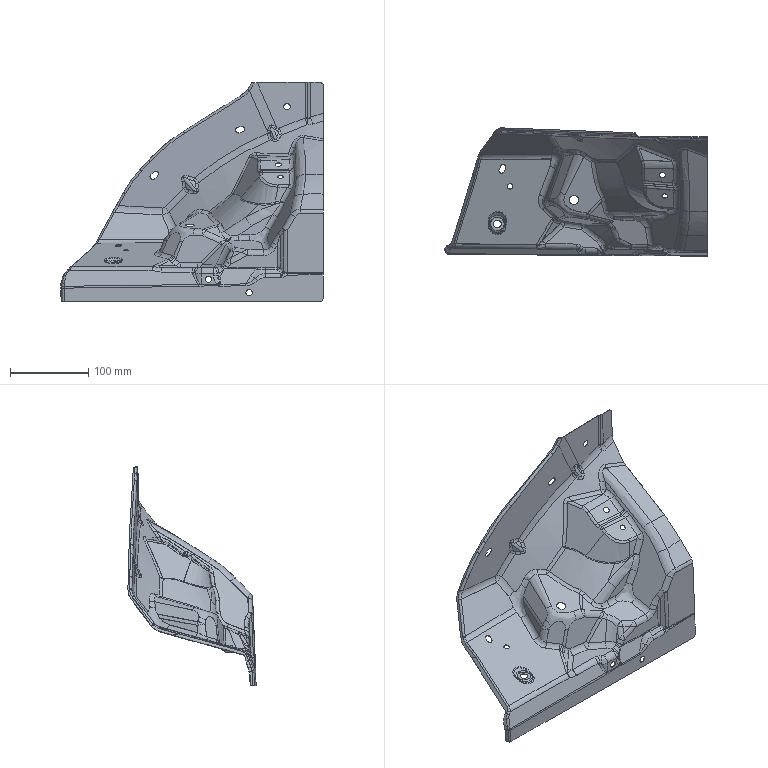Part | 1 solid | 678 faces | box 336.403 x 163.981 x 280.945 mm | volume 81231 mm3 | spline 397 | cylinder 184 | plane 86 | sphere 8 | other 3 | commonest cylinder face diameters 16 x29 17.6 x16 10 x13 14.4 x13 20 x12 7 x10